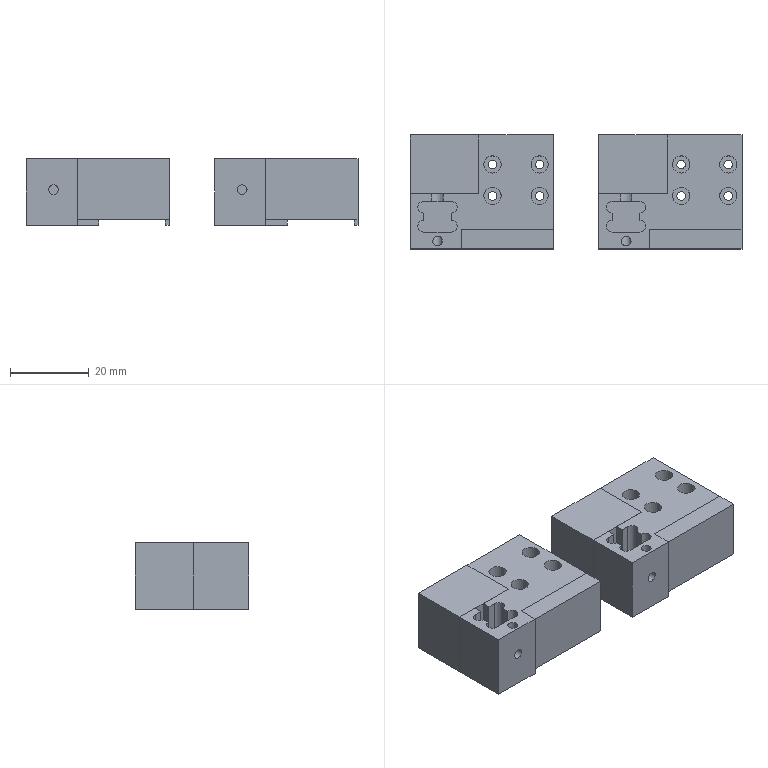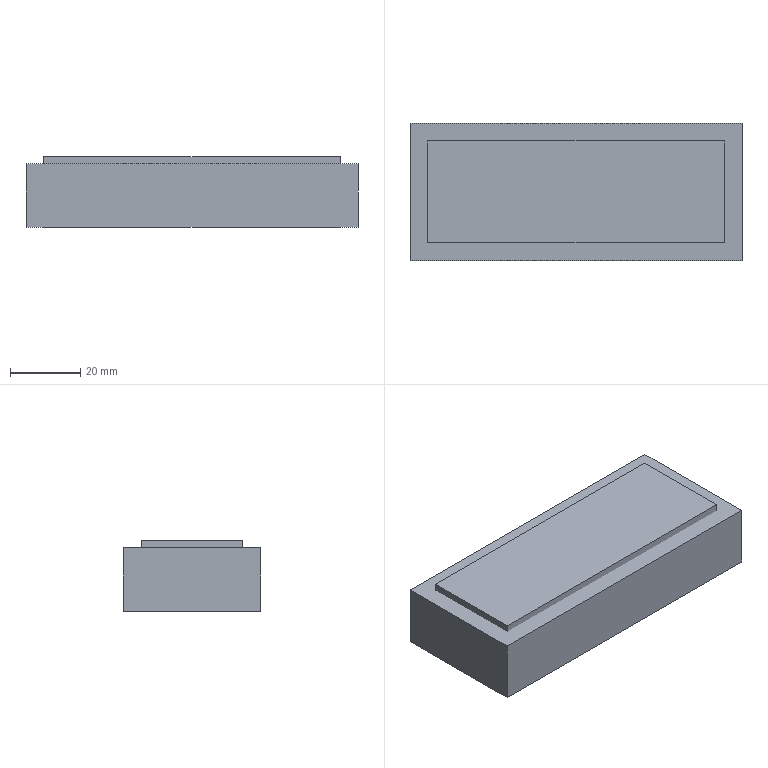CAM job | NX | 3+2 milling, drilling | part box 84.5 x 29 x 17 mm | stock box 94.5 x 39 x 20 mm
Tools:
number,name,description,diameter,corner_radius,flute_length,length,flutes
1,D63,Milling Tool-5 Parameters,63.0,0.0,50.0,75.0,2
10,D10,Milling Tool-5 Parameters,10.0,0.0,50.0,75.0,2
7,D6A45,Milling Tool-5 Parameters,6.0,0.0,50.0,75.0,2
12,2.5ZT,Drilling Tool,2.5,0.0,35.0,50.0,2
14,2.2ZT,Drilling Tool,2.19,0.0,35.0,50.0,2
3,D3,Milling Tool-5 Parameters,3.0,0.0,50.0,75.0,2
13,2.05ZT,Drilling Tool,2.04,0.0,35.0,50.0,2
18,8.0ZT,Drilling Tool,8.0,0.0,35.0,50.0,2
Operations:
program,operation,operation_type,tool,method,geometry_group,spindle_rpm,surface_speed,feed_per_tooth,feed_cut,feed_plunge,cut_length_mm,path_length_mm,cut_time_min,machine_time_min
1,FLOOR_WALL,VolumeBased25DMillingOperation,D63,METHOD,A,6500.0,1286.0,0.1154,1500.0,100.0,169.5,223.5,0.113,0.1184
1,ZLEVEL_PROFILE_1,ZLevelMilling,D10,METHOD,A,9500.0,298.0,0.1579,3000.0,1000.0,5756.839,5927.994,1.983,2
1,ZLEVEL_PROFILE,ZLevelMilling,D10,METHOD,A,9500.0,298.0,0.0789,1500.0,100.0,341.509,574.863,0.2277,0.251
1,DRILLING,Operation,D6A45,METHOD,A,5000.0,94.0,0.025,250.0,0.0,72.0,402.014,0.288,0.321
1,DRILLING_COPY,Operation,2.5ZT,METHOD,A,2000.0,15.0,0.03,120.0,0.0,26.302,163.698,0.2192,0.2329
1,DRILLING_COPY_COPY,Operation,2.2ZT,METHOD,A,2000.0,15.0,0.03,120.0,0.0,165.263,506.567,1.377,1.411
1,HOLE_MILLING,CylinderMilling,D3,METHOD,A,9500.0,89.0,0.0526,1000.0,100.0,2516.899,3192.899,2.517,2.584
1,FLOOR_WALL_1,VolumeBased25DMillingOperation,D3,METHOD,A,9500.0,89.0,0.0658,1250.0,100.0,6962.606,7338.238,5.57,5.608
1,PLANAR_MILL,PlanarMilling,D6A45,METHOD,A,9500.0,179.0,0.0658,1250.0,100.0,501.586,1340.519,0.4013,0.4852
2,FLOOR_WALL_COPY,VolumeBased25DMillingOperation,D63,METHOD,B,6500.0,1286.0,0.1154,1500.0,100.0,490.5,961.501,0.327,0.3741
2,FLOOR_WALL_1_COPY_1_COPY_COPY,VolumeBased25DMillingOperation,D10,METHOD,B,9500.0,119.0,0.1316,2500.0,1000.0,509.095,692.562,0.2095,0.2278
2,PLANAR_MILL_COPY,PlanarMilling,D6A45,METHOD,B,9500.0,179.0,0.0658,1250.0,100.0,342.056,632.121,0.2736,0.3027
2,PLANAR_MILL_COPY_COPY,PlanarMilling,D6A45,METHOD,B,9500.0,179.0,0.0658,1250.0,100.0,82.734,432.504,0.0662,0.1012
2,刀补10,VolumeBased25DMillingOperation,D10,METHOD,B,9500.0,119.0,0.0632,1200.0,1000.0,162.073,337.148,0.1363,0.1538
3,DRILLING_COPY_1,Operation,D6A45,METHOD,C,5000.0,94.0,0.025,250.0,0.0,17.4,133.625,0.0696,0.0812
3,DRILLING_COPY_COPY_COPY,Operation,2.05ZT,METHOD,C,2000.0,15.0,0.03,120.0,0.0,24.348,137.497,0.2029,0.2142
3,DRILLING_COPY_COPY_COPY_COPY,Operation,8.0ZT,METHOD,C,2000.0,50.0,0.0625,250.0,0.0,30.903,121.807,0.1236,0.1327
3,FLOOR_WALL_1_1,VolumeBased25DMillingOperation,D10,METHOD,C,9500.0,298.0,0.1316,2500.0,1000.0,1001.5,1085.1,0.4042,0.4126
3,FLOOR_WALL_1_COPY_COPY_COPY_2,VolumeBased25DMillingOperation,D10,METHOD,C,9500.0,298.0,0.0789,1500.0,1000.0,126.856,232.692,0.0866,0.0972
3,HOLE_MILLING_1,CylinderMilling,D3,METHOD,C,9500.0,89.0,0.0658,1250.0,100.0,44.062,135.362,0.0352,0.0444
3,PLANAR_PROFILE,PlanarMilling,D3,METHOD,C,9500.0,89.0,0.0658,1250.0,100.0,218.08,1587.582,0.1745,0.3114
3,PLANAR_MILL_COPY_2_COPY,PlanarMilling,D6A45,METHOD,C,9500.0,179.0,0.0658,1250.0,100.0,136.513,456.514,0.1092,0.1412
3,PLANAR_MILL_COPY_2_COPY_COPY,PlanarMilling,D6A45,METHOD,C,9500.0,179.0,0.0658,1250.0,100.0,76.668,162.468,0.0613,0.0699
4,DRILLING_COPY_1_COPY,Operation,D6A45,METHOD,D,5000.0,94.0,0.025,250.0,0.0,4.35,68.7,0.0174,0.0238
4,DRILLING_COPY_COPY_1,Operation,2.5ZT,METHOD,D,2000.0,15.0,0.03,120.0,0.0,9.551,79.102,0.0796,0.0865
4,FLOOR_WALL_1_1_COPY,VolumeBased25DMillingOperation,D10,METHOD,D,9500.0,298.0,0.1316,2500.0,1000.0,1313.022,1376.822,0.5288,0.5352
4,FLOOR_WALL_1_COPY_COPY_COPY_2_COPY,VolumeBased25DMillingOperation,D10,METHOD,D,9500.0,298.0,0.0789,1500.0,1000.0,189.258,268.758,0.1277,0.1357
4,PLANAR_MILL_COPY_2_COPY_COPY_1,PlanarMilling,D6A45,METHOD,D,9500.0,179.0,0.0658,1250.0,100.0,82.472,201.936,0.066,0.0779
4,PLANAR_MILL_COPY_2_COPY_COPY_1_COPY,PlanarMilling,D6A45,METHOD,D,9500.0,179.0,0.0658,1250.0,100.0,100.693,249.679,0.0806,0.0955